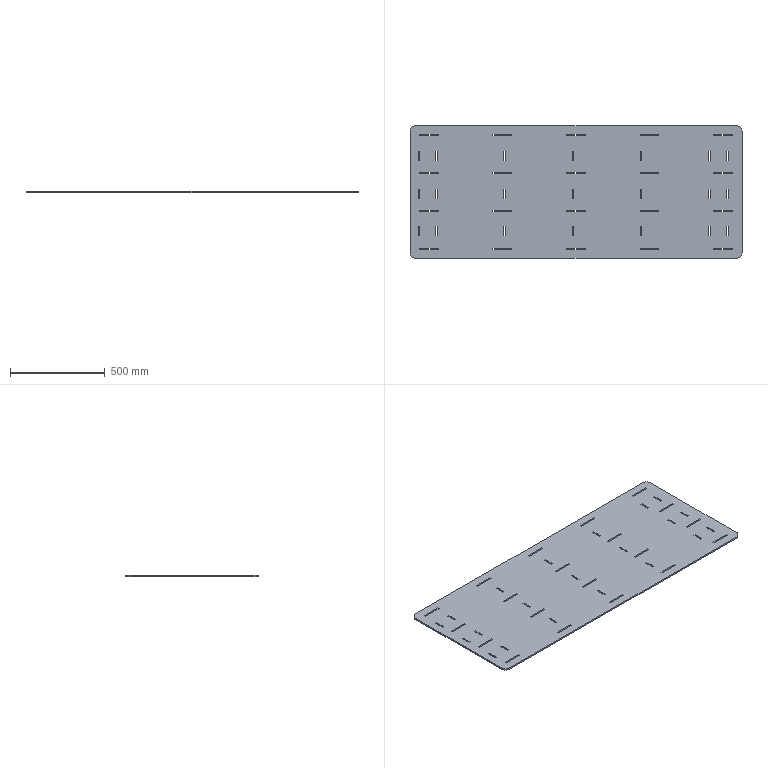Part | SolidWorks | features FlatPattern 1, SMBaseFlange 1, SheetMetal 1 | 1 solid | 174 faces | box 1750 x 700 x 8 mm | volume 9598619 mm3 | plane 170 | cylinder 4 | commonest cylinder face diameters 60 x4